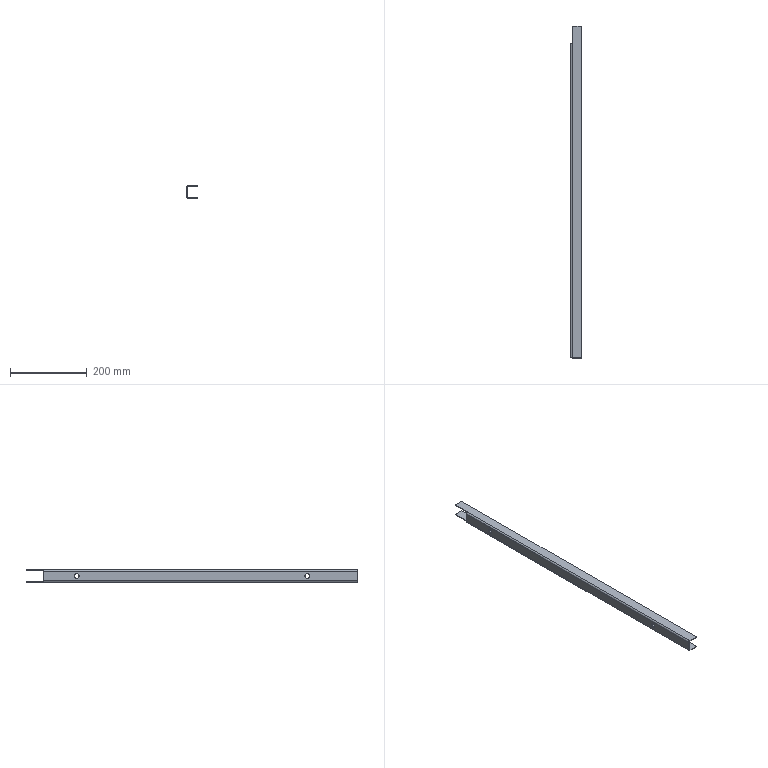Part | NX | features solid 2 | 1 solid | 28 faces | box 28 x 864.5 x 32 mm | volume 136877 mm3 | cylinder 14 | plane 14 | commonest cylinder face diameters 8 x8 12 x4 4 x2
STEP:
#1=CARTESIAN_POINT('',(1130.,-1461.75,470.));
#2=VERTEX_POINT('',#1);
#3=CARTESIAN_POINT('',(1130.,-1461.75,472.));
#4=VERTEX_POINT('',#3);
#5=CARTESIAN_POINT('',(1130.,-1461.75,1335.545));
#6=DIRECTION('',(0.,0.,-1.));
#7=VECTOR('',#6,1000.);
#8=LINE('',#5,#7);
#9=EDGE_CURVE('',#2,#4,#8,.F.);
#10=ORIENTED_EDGE('',*,*,#9,.T.);
#11=CARTESIAN_POINT('',(1130.,-1453.75,472.));
#12=VERTEX_POINT('',#11);
#13=CARTESIAN_POINT('',(1130.,-1457.75,472.));
#14=DIRECTION('',(0.,0.,-1.));
#15=DIRECTION('',(0.,1.,0.));
#16=AXIS2_PLACEMENT_3D('',#13,#14,#15);
#17=CIRCLE('',#16,4.);
#18=EDGE_CURVE('',#12,#4,#17,.T.);
#19=ORIENTED_EDGE('',*,*,#18,.F.);
#20=CARTESIAN_POINT('',(1130.,-1453.75,470.));
#21=VERTEX_POINT('',#20);
#22=CARTESIAN_POINT('',(1130.,-1453.75,1335.545));
#23=DIRECTION('',(0.,0.,-1.));
#24=VECTOR('',#23,1000.);
#25=LINE('',#22,#24);
#26=EDGE_CURVE('',#12,#21,#25,.T.);
#27=ORIENTED_EDGE('',*,*,#26,.T.);
#28=CARTESIAN_POINT('',(1130.,-1457.75,470.));
#29=DIRECTION('',(0.,0.,-1.));
#30=DIRECTION('',(0.,1.,0.));
#31=AXIS2_PLACEMENT_3D('',#28,#29,#30);
#32=CIRCLE('',#31,4.);
#33=EDGE_CURVE('',#21,#2,#32,.T.);
#34=ORIENTED_EDGE('',*,*,#33,.T.);
#35=EDGE_LOOP('',(#10,#19,#27,#34));
#36=FACE_BOUND('',#35,.T.);
#37=CARTESIAN_POINT('',(1130.,-1457.75,1335.545));
#38=DIRECTION('',(0.,0.,-1.));
#39=DIRECTION('',(0.,1.,0.));
#40=AXIS2_PLACEMENT_3D('',#37,#38,#39);
#41=CYLINDRICAL_SURFACE('',#40,4.);
#42=ADVANCED_FACE('',(#36),#41,.F.);
#43=CARTESIAN_POINT('',(1130.,-761.75,470.));
#44=VERTEX_POINT('',#43);
#45=CARTESIAN_POINT('',(1130.,-761.75,472.));
#46=VERTEX_POINT('',#45);
#47=CARTESIAN_POINT('',(1130.,-761.75,1335.545));
#48=DIRECTION('',(0.,0.,-1.));
#49=VECTOR('',#48,1000.);
#50=LINE('',#47,#49);
#51=EDGE_CURVE('',#44,#46,#50,.F.);
#52=ORIENTED_EDGE('',*,*,#51,.T.);
#53=CARTESIAN_POINT('',(1130.,-753.75,472.));
#54=VERTEX_POINT('',#53);
#55=CARTESIAN_POINT('',(1130.,-757.75,472.));
#56=DIRECTION('',(0.,0.,-1.));
#57=DIRECTION('',(0.,1.,0.));
#58=AXIS2_PLACEMENT_3D('',#55,#56,#57);
#59=CIRCLE('',#58,4.);
#60=EDGE_CURVE('',#54,#46,#59,.T.);
#61=ORIENTED_EDGE('',*,*,#60,.F.);
#62=CARTESIAN_POINT('',(1130.,-753.75,470.));
#63=VERTEX_POINT('',#62);
#64=CARTESIAN_POINT('',(1130.,-753.75,1335.545));
#65=DIRECTION('',(0.,0.,-1.));
#66=VECTOR('',#65,1000.);
#67=LINE('',#64,#66);
#68=EDGE_CURVE('',#54,#63,#67,.T.);
#69=ORIENTED_EDGE('',*,*,#68,.T.);
#70=CARTESIAN_POINT('',(1130.,-757.75,470.));
#71=DIRECTION('',(0.,0.,-1.));
#72=DIRECTION('',(0.,1.,0.));
#73=AXIS2_PLACEMENT_3D('',#70,#71,#72);
#74=CIRCLE('',#73,4.);
#75=EDGE_CURVE('',#63,#44,#74,.T.);
#76=ORIENTED_EDGE('',*,*,#75,.T.);
#77=EDGE_LOOP('',(#52,#61,#69,#76));
#78=FACE_BOUND('',#77,.T.);
#79=CARTESIAN_POINT('',(1130.,-757.75,1335.545));
#80=DIRECTION('',(0.,0.,-1.));
#81=DIRECTION('',(0.,1.,0.));
#82=AXIS2_PLACEMENT_3D('',#79,#80,#81);
#83=CYLINDRICAL_SURFACE('',#82,4.);
#84=ADVANCED_FACE('',(#78),#83,.F.);
#85=CARTESIAN_POINT('',(1130.,-1111.75,470.));
#86=VERTEX_POINT('',#85);
#87=CARTESIAN_POINT('',(1130.,-1111.75,472.));
#88=VERTEX_POINT('',#87);
#89=CARTESIAN_POINT('',(1130.,-1111.75,1335.545));
#90=DIRECTION('',(0.,0.,-1.));
#91=VECTOR('',#90,1000.);
#92=LINE('',#89,#91);
#93=EDGE_CURVE('',#86,#88,#92,.F.);
#94=ORIENTED_EDGE('',*,*,#93,.T.);
#95=CARTESIAN_POINT('',(1130.,-1103.75,472.));
#96=VERTEX_POINT('',#95);
#97=CARTESIAN_POINT('',(1130.,-1107.75,472.));
#98=DIRECTION('',(0.,0.,-1.));
#99=DIRECTION('',(0.,1.,0.));
#100=AXIS2_PLACEMENT_3D('',#97,#98,#99);
#101=CIRCLE('',#100,4.);
#102=EDGE_CURVE('',#96,#88,#101,.T.);
#103=ORIENTED_EDGE('',*,*,#102,.F.);
#104=CARTESIAN_POINT('',(1130.,-1103.75,470.));
#105=VERTEX_POINT('',#104);
#106=CARTESIAN_POINT('',(1130.,-1103.75,1335.545));
#107=DIRECTION('',(0.,0.,-1.));
#108=VECTOR('',#107,1000.);
#109=LINE('',#106,#108);
#110=EDGE_CURVE('',#96,#105,#109,.T.);
#111=ORIENTED_EDGE('',*,*,#110,.T.);
#112=CARTESIAN_POINT('',(1130.,-1107.75,470.));
#113=DIRECTION('',(0.,0.,-1.));
#114=DIRECTION('',(0.,1.,0.));
#115=AXIS2_PLACEMENT_3D('',#112,#113,#114);
#116=CIRCLE('',#115,4.);
#117=EDGE_CURVE('',#105,#86,#116,.T.);
#118=ORIENTED_EDGE('',*,*,#117,.T.);
#119=EDGE_LOOP('',(#94,#103,#111,#118));
#120=FACE_BOUND('',#119,.T.);
#121=CARTESIAN_POINT('',(1130.,-1107.75,1335.545));
#122=DIRECTION('',(0.,0.,-1.));
#123=DIRECTION('',(0.,1.,0.));
#124=AXIS2_PLACEMENT_3D('',#121,#122,#123);
#125=CYLINDRICAL_SURFACE('',#124,4.);
#126=ADVANCED_FACE('',(#120),#125,.F.);
#127=CARTESIAN_POINT('',(1110.,-807.75,492.));
#128=VERTEX_POINT('',#127);
#129=CARTESIAN_POINT('',(1112.,-807.75,492.));
#130=VERTEX_POINT('',#129);
#131=CARTESIAN_POINT('',(1975.545,-807.75,492.));
#132=DIRECTION('',(-1.,0.,0.));
#133=VECTOR('',#132,1000.);
#134=LINE('',#131,#133);
#135=EDGE_CURVE('',#128,#130,#134,.F.);
#136=ORIENTED_EDGE('',*,*,#135,.T.);
#137=CARTESIAN_POINT('',(1112.,-807.75,480.));
#138=VERTEX_POINT('',#137);
#139=CARTESIAN_POINT('',(1112.,-807.75,486.));
#140=DIRECTION('',(-1.,0.,0.));
#141=DIRECTION('',(0.,0.,-1.));
#142=AXIS2_PLACEMENT_3D('',#139,#140,#141);
#143=CIRCLE('',#142,6.);
#144=EDGE_CURVE('',#138,#130,#143,.T.);
#145=ORIENTED_EDGE('',*,*,#144,.F.);
#146=CARTESIAN_POINT('',(1110.,-807.75,480.));
#147=VERTEX_POINT('',#146);
#148=CARTESIAN_POINT('',(1975.545,-807.75,480.));
#149=DIRECTION('',(-1.,0.,0.));
#150=VECTOR('',#149,1000.);
#151=LINE('',#148,#150);
#152=EDGE_CURVE('',#138,#147,#151,.T.);
#153=ORIENTED_EDGE('',*,*,#152,.T.);
#154=CARTESIAN_POINT('',(1110.,-807.75,486.));
#155=DIRECTION('',(-1.,0.,0.));
#156=DIRECTION('',(0.,-1.,0.));
#157=AXIS2_PLACEMENT_3D('',#154,#155,#156);
#158=CIRCLE('',#157,6.);
#159=EDGE_CURVE('',#147,#128,#158,.T.);
#160=ORIENTED_EDGE('',*,*,#159,.T.);
#161=EDGE_LOOP('',(#136,#145,#153,#160));
#162=FACE_BOUND('',#161,.T.);
#163=CARTESIAN_POINT('',(1975.545,-807.75,486.));
#164=DIRECTION('',(-1.,0.,0.));
#165=DIRECTION('',(0.,0.,-1.));
#166=AXIS2_PLACEMENT_3D('',#163,#164,#165);
#167=CYLINDRICAL_SURFACE('',#166,6.);
#168=ADVANCED_FACE('',(#162),#167,.F.);
#169=CARTESIAN_POINT('',(1112.,-1407.75,492.));
#170=VERTEX_POINT('',#169);
#171=CARTESIAN_POINT('',(1110.,-1407.75,492.));
#172=VERTEX_POINT('',#171);
#173=CARTESIAN_POINT('',(1975.545,-1407.75,492.));
#174=DIRECTION('',(-1.,0.,0.));
#175=VECTOR('',#174,1000.);
#176=LINE('',#173,#175);
#177=EDGE_CURVE('',#170,#172,#176,.T.);
#178=ORIENTED_EDGE('',*,*,#177,.F.);
#179=CARTESIAN_POINT('',(1112.,-1407.75,480.));
#180=VERTEX_POINT('',#179);
#181=CARTESIAN_POINT('',(1112.,-1407.75,486.));
#182=DIRECTION('',(-1.,0.,0.));
#183=DIRECTION('',(0.,0.,-1.));
#184=AXIS2_PLACEMENT_3D('',#181,#182,#183);
#185=CIRCLE('',#184,6.);
#186=EDGE_CURVE('',#180,#170,#185,.T.);
#187=ORIENTED_EDGE('',*,*,#186,.F.);
#188=CARTESIAN_POINT('',(1110.,-1407.75,480.));
#189=VERTEX_POINT('',#188);
#190=CARTESIAN_POINT('',(1975.545,-1407.75,480.));
#191=DIRECTION('',(-1.,0.,0.));
#192=VECTOR('',#191,1000.);
#193=LINE('',#190,#192);
#194=EDGE_CURVE('',#189,#180,#193,.F.);
#195=ORIENTED_EDGE('',*,*,#194,.F.);
#196=CARTESIAN_POINT('',(1110.,-1407.75,486.));
#197=DIRECTION('',(-1.,0.,0.));
#198=DIRECTION('',(0.,-1.,0.));
#199=AXIS2_PLACEMENT_3D('',#196,#197,#198);
#200=CIRCLE('',#199,6.);
#201=EDGE_CURVE('',#189,#172,#200,.T.);
#202=ORIENTED_EDGE('',*,*,#201,.T.);
#203=EDGE_LOOP('',(#178,#187,#195,#202));
#204=FACE_BOUND('',#203,.T.);
#205=CARTESIAN_POINT('',(1975.545,-1407.75,486.));
#206=DIRECTION('',(-1.,0.,0.));
#207=DIRECTION('',(0.,0.,-1.));
#208=AXIS2_PLACEMENT_3D('',#205,#206,#207);
#209=CYLINDRICAL_SURFACE('',#208,6.);
#210=ADVANCED_FACE('',(#204),#209,.F.);
#211=CARTESIAN_POINT('',(1114.,-720.,500.));
#212=VERTEX_POINT('',#211);
#213=CARTESIAN_POINT('',(1112.,-720.,498.));
#214=VERTEX_POINT('',#213);
#215=CARTESIAN_POINT('',(1114.,-720.,498.));
#216=DIRECTION('',(0.,-1.,0.));
#217=DIRECTION('',(0.,0.,-1.));
#218=AXIS2_PLACEMENT_3D('',#215,#216,#217);
#219=CIRCLE('',#218,2.);
#220=EDGE_CURVE('',#212,#214,#219,.T.);
#221=ORIENTED_EDGE('',*,*,#220,.T.);
#222=CARTESIAN_POINT('',(1112.,-720.,474.));
#223=VERTEX_POINT('',#222);
#224=CARTESIAN_POINT('',(1112.,-720.,502.));
#225=DIRECTION('',(0.,0.,-1.));
#226=VECTOR('',#225,1000.);
#227=LINE('',#224,#226);
#228=EDGE_CURVE('',#214,#223,#227,.T.);
#229=ORIENTED_EDGE('',*,*,#228,.T.);
#230=CARTESIAN_POINT('',(1114.,-720.,472.));
#231=VERTEX_POINT('',#230);
#232=CARTESIAN_POINT('',(1114.,-720.,474.));
#233=DIRECTION('',(0.,-1.,0.));
#234=DIRECTION('',(0.,0.,-1.));
#235=AXIS2_PLACEMENT_3D('',#232,#233,#234);
#236=CIRCLE('',#235,2.);
#237=EDGE_CURVE('',#223,#231,#236,.T.);
#238=ORIENTED_EDGE('',*,*,#237,.T.);
#239=CARTESIAN_POINT('',(1115.,-720.,472.));
#240=VERTEX_POINT('',#239);
#241=CARTESIAN_POINT('',(1110.,-720.,472.));
#242=DIRECTION('',(1.,0.,0.));
#243=VECTOR('',#242,1000.);
#244=LINE('',#241,#243);
#245=EDGE_CURVE('',#231,#240,#244,.T.);
#246=ORIENTED_EDGE('',*,*,#245,.T.);
#247=CARTESIAN_POINT('',(1115.,-720.,470.));
#248=VERTEX_POINT('',#247);
#249=CARTESIAN_POINT('',(1115.,-720.,470.));
#250=DIRECTION('',(0.,0.,-1.));
#251=VECTOR('',#250,1000.);
#252=LINE('',#249,#251);
#253=EDGE_CURVE('',#240,#248,#252,.T.);
#254=ORIENTED_EDGE('',*,*,#253,.T.);
#255=CARTESIAN_POINT('',(1114.,-720.,470.));
#256=VERTEX_POINT('',#255);
#257=CARTESIAN_POINT('',(1110.,-720.,470.));
#258=DIRECTION('',(1.,0.,0.));
#259=VECTOR('',#258,1000.);
#260=LINE('',#257,#259);
#261=EDGE_CURVE('',#256,#248,#260,.T.);
#262=ORIENTED_EDGE('',*,*,#261,.F.);
#263=CARTESIAN_POINT('',(1110.,-720.,474.));
#264=VERTEX_POINT('',#263);
#265=CARTESIAN_POINT('',(1114.,-720.,474.));
#266=DIRECTION('',(0.,-1.,0.));
#267=DIRECTION('',(0.,0.,1.));
#268=AXIS2_PLACEMENT_3D('',#265,#266,#267);
#269=CIRCLE('',#268,4.);
#270=EDGE_CURVE('',#264,#256,#269,.T.);
#271=ORIENTED_EDGE('',*,*,#270,.F.);
#272=CARTESIAN_POINT('',(1110.,-720.,498.));
#273=VERTEX_POINT('',#272);
#274=CARTESIAN_POINT('',(1110.,-720.,502.));
#275=DIRECTION('',(0.,0.,-1.));
#276=VECTOR('',#275,1000.);
#277=LINE('',#274,#276);
#278=EDGE_CURVE('',#273,#264,#277,.T.);
#279=ORIENTED_EDGE('',*,*,#278,.F.);
#280=CARTESIAN_POINT('',(1114.,-720.,502.));
#281=VERTEX_POINT('',#280);
#282=CARTESIAN_POINT('',(1114.,-720.,498.));
#283=DIRECTION('',(0.,-1.,0.));
#284=DIRECTION('',(0.,0.,1.));
#285=AXIS2_PLACEMENT_3D('',#282,#283,#284);
#286=CIRCLE('',#285,4.);
#287=EDGE_CURVE('',#281,#273,#286,.T.);
#288=ORIENTED_EDGE('',*,*,#287,.F.);
#289=CARTESIAN_POINT('',(1115.,-720.,502.));
#290=VERTEX_POINT('',#289);
#291=CARTESIAN_POINT('',(1138.,-720.,502.));
#292=DIRECTION('',(-1.,0.,0.));
#293=VECTOR('',#292,1000.);
#294=LINE('',#291,#293);
#295=EDGE_CURVE('',#290,#281,#294,.T.);
#296=ORIENTED_EDGE('',*,*,#295,.F.);
#297=CARTESIAN_POINT('',(1115.,-720.,500.));
#298=VERTEX_POINT('',#297);
#299=CARTESIAN_POINT('',(1115.,-720.,502.));
#300=DIRECTION('',(0.,0.,1.));
#301=VECTOR('',#300,1000.);
#302=LINE('',#299,#301);
#303=EDGE_CURVE('',#298,#290,#302,.T.);
#304=ORIENTED_EDGE('',*,*,#303,.F.);
#305=CARTESIAN_POINT('',(1138.,-720.,500.));
#306=DIRECTION('',(-1.,0.,0.));
#307=VECTOR('',#306,1000.);
#308=LINE('',#305,#307);
#309=EDGE_CURVE('',#298,#212,#308,.T.);
#310=ORIENTED_EDGE('',*,*,#309,.T.);
#311=EDGE_LOOP('',(#221,#229,#238,#246,#254,#262,#271,#279,#288,#296,#304,#310));
#312=FACE_BOUND('',#311,.T.);
#313=CARTESIAN_POINT('',(1114.,-720.,498.));
#314=DIRECTION('',(0.,-1.,0.));
#315=DIRECTION('',(-1.,0.,0.));
#316=AXIS2_PLACEMENT_3D('',#313,#314,#315);
#317=PLANE('',#316);
#318=ADVANCED_FACE('',(#312),#317,.F.);
#319=CARTESIAN_POINT('',(1115.,-675.5,472.));
#320=VERTEX_POINT('',#319);
#321=CARTESIAN_POINT('',(1115.,-675.5,470.));
#322=VERTEX_POINT('',#321);
#323=CARTESIAN_POINT('',(1115.,-675.5,470.));
#324=DIRECTION('',(0.,0.,-1.));
#325=VECTOR('',#324,1000.);
#326=LINE('',#323,#325);
#327=EDGE_CURVE('',#320,#322,#326,.T.);
#328=ORIENTED_EDGE('',*,*,#327,.T.);
#329=CARTESIAN_POINT('',(1115.,-675.5,470.));
#330=DIRECTION('',(0.,1.,0.));
#331=VECTOR('',#330,1000.);
#332=LINE('',#329,#331);
#333=EDGE_CURVE('',#248,#322,#332,.T.);
#334=ORIENTED_EDGE('',*,*,#333,.F.);
#335=ORIENTED_EDGE('',*,*,#253,.F.);
#336=CARTESIAN_POINT('',(1115.,-675.5,472.));
#337=DIRECTION('',(0.,1.,0.));
#338=VECTOR('',#337,1000.);
#339=LINE('',#336,#338);
#340=EDGE_CURVE('',#240,#320,#339,.T.);
#341=ORIENTED_EDGE('',*,*,#340,.T.);
#342=EDGE_LOOP('',(#328,#334,#335,#341));
#343=FACE_BOUND('',#342,.T.);
#344=CARTESIAN_POINT('',(1115.,-675.5,470.));
#345=DIRECTION('',(-1.,0.,0.));
#346=DIRECTION('',(0.,0.,1.));
#347=AXIS2_PLACEMENT_3D('',#344,#345,#346);
#348=PLANE('',#347);
#349=ADVANCED_FACE('',(#343),#348,.T.);
#350=ORIENTED_EDGE('',*,*,#303,.T.);
#351=CARTESIAN_POINT('',(1115.,-675.5,502.));
#352=VERTEX_POINT('',#351);
#353=CARTESIAN_POINT('',(1115.,-675.5,502.));
#354=DIRECTION('',(0.,-1.,0.));
#355=VECTOR('',#354,1000.);
#356=LINE('',#353,#355);
#357=EDGE_CURVE('',#352,#290,#356,.T.);
#358=ORIENTED_EDGE('',*,*,#357,.F.);
#359=CARTESIAN_POINT('',(1115.,-675.5,500.));
#360=VERTEX_POINT('',#359);
#361=CARTESIAN_POINT('',(1115.,-675.5,502.));
#362=DIRECTION('',(0.,0.,1.));
#363=VECTOR('',#362,1000.);
#364=LINE('',#361,#363);
#365=EDGE_CURVE('',#360,#352,#364,.T.);
#366=ORIENTED_EDGE('',*,*,#365,.F.);
#367=CARTESIAN_POINT('',(1115.,-675.5,500.));
#368=DIRECTION('',(0.,-1.,0.));
#369=VECTOR('',#368,1000.);
#370=LINE('',#367,#369);
#371=EDGE_CURVE('',#360,#298,#370,.T.);
#372=ORIENTED_EDGE('',*,*,#371,.T.);
#373=EDGE_LOOP('',(#350,#358,#366,#372));
#374=FACE_BOUND('',#373,.T.);
#375=CARTESIAN_POINT('',(1115.,-675.5,502.));
#376=DIRECTION('',(-1.,0.,0.));
#377=DIRECTION('',(0.,0.,1.));
#378=AXIS2_PLACEMENT_3D('',#375,#376,#377);
#379=PLANE('',#378);
#380=ADVANCED_FACE('',(#374),#379,.T.);
#381=ORIENTED_EDGE('',*,*,#102,.T.);
#382=CARTESIAN_POINT('',(1130.,-1107.75,472.));
#383=DIRECTION('',(0.,0.,-1.));
#384=DIRECTION('',(0.,1.,0.));
#385=AXIS2_PLACEMENT_3D('',#382,#383,#384);
#386=CIRCLE('',#385,4.);
#387=EDGE_CURVE('',#88,#96,#386,.T.);
#388=ORIENTED_EDGE('',*,*,#387,.T.);
#389=EDGE_LOOP('',(#381,#388));
#390=FACE_BOUND('',#389,.T.);
#391=ORIENTED_EDGE('',*,*,#60,.T.);
#392=CARTESIAN_POINT('',(1130.,-757.75,472.));
#393=DIRECTION('',(0.,0.,-1.));
#394=DIRECTION('',(0.,1.,0.));
#395=AXIS2_PLACEMENT_3D('',#392,#393,#394);
#396=CIRCLE('',#395,4.);
#397=EDGE_CURVE('',#46,#54,#396,.T.);
#398=ORIENTED_EDGE('',*,*,#397,.T.);
#399=EDGE_LOOP('',(#391,#398));
#400=FACE_BOUND('',#399,.T.);
#401=ORIENTED_EDGE('',*,*,#18,.T.);
#402=CARTESIAN_POINT('',(1130.,-1457.75,472.));
#403=DIRECTION('',(0.,0.,-1.));
#404=DIRECTION('',(0.,1.,0.));
#405=AXIS2_PLACEMENT_3D('',#402,#403,#404);
#406=CIRCLE('',#405,4.);
#407=EDGE_CURVE('',#4,#12,#406,.T.);
#408=ORIENTED_EDGE('',*,*,#407,.T.);
#409=EDGE_LOOP('',(#401,#408));
#410=FACE_BOUND('',#409,.T.);
#411=CARTESIAN_POINT('',(1138.,-675.5,472.));
#412=VERTEX_POINT('',#411);
#413=CARTESIAN_POINT('',(1110.,-675.5,472.));
#414=DIRECTION('',(1.,0.,0.));
#415=VECTOR('',#414,1000.);
#416=LINE('',#413,#415);
#417=EDGE_CURVE('',#320,#412,#416,.T.);
#418=ORIENTED_EDGE('',*,*,#417,.F.);
#419=ORIENTED_EDGE('',*,*,#340,.F.);
#420=ORIENTED_EDGE('',*,*,#245,.F.);
#421=CARTESIAN_POINT('',(1114.,-1540.,472.));
#422=VERTEX_POINT('',#421);
#423=CARTESIAN_POINT('',(1114.,-675.5,472.));
#424=DIRECTION('',(0.,-1.,0.));
#425=VECTOR('',#424,1000.);
#426=LINE('',#423,#425);
#427=EDGE_CURVE('',#231,#422,#426,.T.);
#428=ORIENTED_EDGE('',*,*,#427,.T.);
#429=CARTESIAN_POINT('',(1138.,-1540.,472.));
#430=VERTEX_POINT('',#429);
#431=CARTESIAN_POINT('',(1110.,-1540.,472.));
#432=DIRECTION('',(1.,0.,0.));
#433=VECTOR('',#432,1000.);
#434=LINE('',#431,#433);
#435=EDGE_CURVE('',#422,#430,#434,.T.);
#436=ORIENTED_EDGE('',*,*,#435,.T.);
#437=CARTESIAN_POINT('',(1138.,-675.5,472.));
#438=DIRECTION('',(0.,-1.,0.));
#439=VECTOR('',#438,1000.);
#440=LINE('',#437,#439);
#441=EDGE_CURVE('',#412,#430,#440,.T.);
#442=ORIENTED_EDGE('',*,*,#441,.F.);
#443=EDGE_LOOP('',(#418,#419,#420,#428,#436,#442));
#444=FACE_BOUND('',#443,.T.);
#445=CARTESIAN_POINT('',(1110.,-675.5,472.));
#446=DIRECTION('',(0.,0.,-1.));
#447=DIRECTION('',(0.,-1.,0.));
#448=AXIS2_PLACEMENT_3D('',#445,#446,#447);
#449=PLANE('',#448);
#450=ADVANCED_FACE('',(#390,#400,#410,#444),#449,.F.);
#451=ORIENTED_EDGE('',*,*,#427,.F.);
#452=ORIENTED_EDGE('',*,*,#237,.F.);
#453=CARTESIAN_POINT('',(1112.,-1540.,474.));
#454=VERTEX_POINT('',#453);
#455=CARTESIAN_POINT('',(1112.,-675.5,474.));
#456=DIRECTION('',(0.,-1.,0.));
#457=VECTOR('',#456,1000.);
#458=LINE('',#455,#457);
#459=EDGE_CURVE('',#223,#454,#458,.T.);
#460=ORIENTED_EDGE('',*,*,#459,.T.);
#461=CARTESIAN_POINT('',(1114.,-1540.,474.));
#462=DIRECTION('',(0.,-1.,0.));
#463=DIRECTION('',(0.,0.,-1.));
#464=AXIS2_PLACEMENT_3D('',#461,#462,#463);
#465=CIRCLE('',#464,2.);
#466=EDGE_CURVE('',#454,#422,#465,.T.);
#467=ORIENTED_EDGE('',*,*,#466,.T.);
#468=EDGE_LOOP('',(#451,#452,#460,#467));
#469=FACE_BOUND('',#468,.T.);
#470=CARTESIAN_POINT('',(1114.,-675.5,474.));
#471=DIRECTION('',(0.,-1.,0.));
#472=DIRECTION('',(0.,0.,-1.));
#473=AXIS2_PLACEMENT_3D('',#470,#471,#472);
#474=CYLINDRICAL_SURFACE('',#473,2.);
#475=ADVANCED_FACE('',(#469),#474,.F.);
#476=ORIENTED_EDGE('',*,*,#186,.T.);
#477=CARTESIAN_POINT('',(1112.,-1407.75,486.));
#478=DIRECTION('',(-1.,0.,0.));
#479=DIRECTION('',(0.,0.,-1.));
#480=AXIS2_PLACEMENT_3D('',#477,#478,#479);
#481=CIRCLE('',#480,6.);
#482=EDGE_CURVE('',#170,#180,#481,.T.);
#483=ORIENTED_EDGE('',*,*,#482,.T.);
#484=EDGE_LOOP('',(#476,#483));
#485=FACE_BOUND('',#484,.T.);
#486=ORIENTED_EDGE('',*,*,#144,.T.);
#487=CARTESIAN_POINT('',(1112.,-807.75,486.));
#488=DIRECTION('',(-1.,0.,0.));
#489=DIRECTION('',(0.,0.,-1.));
#490=AXIS2_PLACEMENT_3D('',#487,#488,#489);
#491=CIRCLE('',#490,6.);
#492=EDGE_CURVE('',#130,#138,#491,.T.);
#493=ORIENTED_EDGE('',*,*,#492,.T.);
#494=EDGE_LOOP('',(#486,#493));
#495=FACE_BOUND('',#494,.T.);
#496=ORIENTED_EDGE('',*,*,#459,.F.);
#497=ORIENTED_EDGE('',*,*,#228,.F.);
#498=CARTESIAN_POINT('',(1112.,-1540.,498.));
#499=VERTEX_POINT('',#498);
#500=CARTESIAN_POINT('',(1112.,-675.5,498.));
#501=DIRECTION('',(0.,-1.,0.));
#502=VECTOR('',#501,1000.);
#503=LINE('',#500,#502);
#504=EDGE_CURVE('',#214,#499,#503,.T.);
#505=ORIENTED_EDGE('',*,*,#504,.T.);
#506=CARTESIAN_POINT('',(1112.,-1540.,502.));
#507=DIRECTION('',(0.,0.,-1.));
#508=VECTOR('',#507,1000.);
#509=LINE('',#506,#508);
#510=EDGE_CURVE('',#499,#454,#509,.T.);
#511=ORIENTED_EDGE('',*,*,#510,.T.);
#512=EDGE_LOOP('',(#496,#497,#505,#511));
#513=FACE_BOUND('',#512,.T.);
#514=CARTESIAN_POINT('',(1112.,-675.5,502.));
#515=DIRECTION('',(-1.,0.,0.));
#516=DIRECTION('',(0.,0.,1.));
#517=AXIS2_PLACEMENT_3D('',#514,#515,#516);
#518=PLANE('',#517);
#519=ADVANCED_FACE('',(#485,#495,#513),#518,.F.);
#520=ORIENTED_EDGE('',*,*,#504,.F.);
#521=ORIENTED_EDGE('',*,*,#220,.F.);
#522=CARTESIAN_POINT('',(1114.,-1540.,500.));
#523=VERTEX_POINT('',#522);
#524=CARTESIAN_POINT('',(1114.,-675.5,500.));
#525=DIRECTION('',(0.,-1.,0.));
#526=VECTOR('',#525,1000.);
#527=LINE('',#524,#526);
#528=EDGE_CURVE('',#212,#523,#527,.T.);
#529=ORIENTED_EDGE('',*,*,#528,.T.);
#530=CARTESIAN_POINT('',(1114.,-1540.,498.));
#531=DIRECTION('',(0.,-1.,0.));
#532=DIRECTION('',(0.,0.,-1.));
#533=AXIS2_PLACEMENT_3D('',#530,#531,#532);
#534=CIRCLE('',#533,2.);
#535=EDGE_CURVE('',#523,#499,#534,.T.);
#536=ORIENTED_EDGE('',*,*,#535,.T.);
#537=EDGE_LOOP('',(#520,#521,#529,#536));
#538=FACE_BOUND('',#537,.T.);
#539=CARTESIAN_POINT('',(1114.,-675.5,498.));
#540=DIRECTION('',(0.,-1.,0.));
#541=DIRECTION('',(0.,0.,-1.));
#542=AXIS2_PLACEMENT_3D('',#539,#540,#541);
#543=CYLINDRICAL_SURFACE('',#542,2.);
#544=ADVANCED_FACE('',(#538),#543,.F.);
#545=ORIENTED_EDGE('',*,*,#309,.F.);
#546=ORIENTED_EDGE('',*,*,#371,.F.);
#547=CARTESIAN_POINT('',(1138.,-675.5,500.));
#548=VERTEX_POINT('',#547);
#549=CARTESIAN_POINT('',(1138.,-675.5,500.));
#550=DIRECTION('',(-1.,0.,0.));
#551=VECTOR('',#550,1000.);
#552=LINE('',#549,#551);
#553=EDGE_CURVE('',#548,#360,#552,.T.);
#554=ORIENTED_EDGE('',*,*,#553,.F.);
#555=CARTESIAN_POINT('',(1138.,-1540.,500.));
#556=VERTEX_POINT('',#555);
#557=CARTESIAN_POINT('',(1138.,-675.5,500.));
#558=DIRECTION('',(0.,-1.,0.));
#559=VECTOR('',#558,1000.);
#560=LINE('',#557,#559);
#561=EDGE_CURVE('',#548,#556,#560,.T.);
#562=ORIENTED_EDGE('',*,*,#561,.T.);
#563=CARTESIAN_POINT('',(1138.,-1540.,500.));
#564=DIRECTION('',(-1.,0.,0.));
#565=VECTOR('',#564,1000.);
#566=LINE('',#563,#565);
#567=EDGE_CURVE('',#556,#523,#566,.T.);
#568=ORIENTED_EDGE('',*,*,#567,.T.);
#569=ORIENTED_EDGE('',*,*,#528,.F.);
#570=EDGE_LOOP('',(#545,#546,#554,#562,#568,#569));
#571=FACE_BOUND('',#570,.T.);
#572=CARTESIAN_POINT('',(1138.,-675.5,500.));
#573=DIRECTION('',(0.,0.,1.));
#574=DIRECTION('',(1.,0.,0.));
#575=AXIS2_PLACEMENT_3D('',#572,#573,#574);
#576=PLANE('',#575);
#577=ADVANCED_FACE('',(#571),#576,.F.);
#578=ORIENTED_EDGE('',*,*,#117,.F.);
#579=CARTESIAN_POINT('',(1130.,-1107.75,470.));
#580=DIRECTION('',(0.,0.,-1.));
#581=DIRECTION('',(0.,1.,0.));
#582=AXIS2_PLACEMENT_3D('',#579,#580,#581);
#583=CIRCLE('',#582,4.);
#584=EDGE_CURVE('',#86,#105,#583,.T.);
#585=ORIENTED_EDGE('',*,*,#584,.F.);
#586=EDGE_LOOP('',(#578,#585));
#587=FACE_BOUND('',#586,.T.);
#588=ORIENTED_EDGE('',*,*,#75,.F.);
#589=CARTESIAN_POINT('',(1130.,-757.75,470.));
#590=DIRECTION('',(0.,0.,-1.));
#591=DIRECTION('',(0.,1.,0.));
#592=AXIS2_PLACEMENT_3D('',#589,#590,#591);
#593=CIRCLE('',#592,4.);
#594=EDGE_CURVE('',#44,#63,#593,.T.);
#595=ORIENTED_EDGE('',*,*,#594,.F.);
#596=EDGE_LOOP('',(#588,#595));
#597=FACE_BOUND('',#596,.T.);
#598=ORIENTED_EDGE('',*,*,#33,.F.);
#599=CARTESIAN_POINT('',(1130.,-1457.75,470.));
#600=DIRECTION('',(0.,0.,-1.));
#601=DIRECTION('',(0.,1.,0.));
#602=AXIS2_PLACEMENT_3D('',#599,#600,#601);
#603=CIRCLE('',#602,4.);
#604=EDGE_CURVE('',#2,#21,#603,.T.);
#605=ORIENTED_EDGE('',*,*,#604,.F.);
#606=EDGE_LOOP('',(#598,#605));
#607=FACE_BOUND('',#606,.T.);
#608=ORIENTED_EDGE('',*,*,#333,.T.);
#609=CARTESIAN_POINT('',(1138.,-675.5,470.));
#610=VERTEX_POINT('',#609);
#611=CARTESIAN_POINT('',(1110.,-675.5,470.));
#612=DIRECTION('',(1.,0.,0.));
#613=VECTOR('',#612,1000.);
#614=LINE('',#611,#613);
#615=EDGE_CURVE('',#322,#610,#614,.T.);
#616=ORIENTED_EDGE('',*,*,#615,.T.);
#617=CARTESIAN_POINT('',(1138.,-1540.,470.));
#618=VERTEX_POINT('',#617);
#619=CARTESIAN_POINT('',(1138.,-675.5,470.));
#620=DIRECTION('',(0.,-1.,0.));
#621=VECTOR('',#620,1000.);
#622=LINE('',#619,#621);
#623=EDGE_CURVE('',#610,#618,#622,.T.);
#624=ORIENTED_EDGE('',*,*,#623,.T.);
#625=CARTESIAN_POINT('',(1114.,-1540.,470.));
#626=VERTEX_POINT('',#625);
#627=CARTESIAN_POINT('',(1110.,-1540.,470.));
#628=DIRECTION('',(1.,0.,0.));
#629=VECTOR('',#628,1000.);
#630=LINE('',#627,#629);
#631=EDGE_CURVE('',#626,#618,#630,.T.);
#632=ORIENTED_EDGE('',*,*,#631,.F.);
#633=CARTESIAN_POINT('',(1114.,-675.5,470.));
#634=DIRECTION('',(0.,-1.,0.));
#635=VECTOR('',#634,1000.);
#636=LINE('',#633,#635);
#637=EDGE_CURVE('',#256,#626,#636,.T.);
#638=ORIENTED_EDGE('',*,*,#637,.F.);
#639=ORIENTED_EDGE('',*,*,#261,.T.);
#640=EDGE_LOOP('',(#608,#616,#624,#632,#638,#639));
#641=FACE_BOUND('',#640,.T.);
#642=CARTESIAN_POINT('',(1110.,-675.5,470.));
#643=DIRECTION('',(0.,0.,-1.));
#644=DIRECTION('',(0.,-1.,0.));
#645=AXIS2_PLACEMENT_3D('',#642,#643,#644);
#646=PLANE('',#645);
#647=ADVANCED_FACE('',(#587,#597,#607,#641),#646,.T.);
#648=ORIENTED_EDGE('',*,*,#270,.T.);
#649=ORIENTED_EDGE('',*,*,#637,.T.);
#650=CARTESIAN_POINT('',(1110.,-1540.,474.));
#651=VERTEX_POINT('',#650);
#652=CARTESIAN_POINT('',(1114.,-1540.,474.));
#653=DIRECTION('',(0.,-1.,0.));
#654=DIRECTION('',(-1.,0.,0.));
#655=AXIS2_PLACEMENT_3D('',#652,#653,#654);
#656=CIRCLE('',#655,4.);
#657=EDGE_CURVE('',#651,#626,#656,.T.);
#658=ORIENTED_EDGE('',*,*,#657,.F.);
#659=CARTESIAN_POINT('',(1110.,-675.5,474.));
#660=DIRECTION('',(0.,-1.,0.));
#661=VECTOR('',#660,1000.);
#662=LINE('',#659,#661);
#663=EDGE_CURVE('',#264,#651,#662,.T.);
#664=ORIENTED_EDGE('',*,*,#663,.F.);
#665=EDGE_LOOP('',(#648,#649,#658,#664));
#666=FACE_BOUND('',#665,.T.);
#667=CARTESIAN_POINT('',(1114.,-675.5,474.));
#668=DIRECTION('',(0.,-1.,0.));
#669=DIRECTION('',(0.,0.,-1.));
#670=AXIS2_PLACEMENT_3D('',#667,#668,#669);
#671=CYLINDRICAL_SURFACE('',#670,4.);
#672=ADVANCED_FACE('',(#666),#671,.T.);
#673=ORIENTED_EDGE('',*,*,#201,.F.);
#674=CARTESIAN_POINT('',(1110.,-1407.75,486.));
#675=DIRECTION('',(-1.,0.,0.));
#676=DIRECTION('',(0.,-1.,0.));
#677=AXIS2_PLACEMENT_3D('',#674,#675,#676);
#678=CIRCLE('',#677,6.);
#679=EDGE_CURVE('',#172,#189,#678,.T.);
#680=ORIENTED_EDGE('',*,*,#679,.F.);
#681=EDGE_LOOP('',(#673,#680));
#682=FACE_BOUND('',#681,.T.);
#683=ORIENTED_EDGE('',*,*,#159,.F.);
#684=CARTESIAN_POINT('',(1110.,-807.75,486.));
#685=DIRECTION('',(-1.,0.,0.));
#686=DIRECTION('',(0.,-1.,0.));
#687=AXIS2_PLACEMENT_3D('',#684,#685,#686);
#688=CIRCLE('',#687,6.);
#689=EDGE_CURVE('',#128,#147,#688,.T.);
#690=ORIENTED_EDGE('',*,*,#689,.F.);
#691=EDGE_LOOP('',(#683,#690));
#692=FACE_BOUND('',#691,.T.);
#693=ORIENTED_EDGE('',*,*,#278,.T.);
#694=ORIENTED_EDGE('',*,*,#663,.T.);
#695=CARTESIAN_POINT('',(1110.,-1540.,498.));
#696=VERTEX_POINT('',#695);
#697=CARTESIAN_POINT('',(1110.,-1540.,502.));
#698=DIRECTION('',(0.,0.,-1.));
#699=VECTOR('',#698,1000.);
#700=LINE('',#697,#699);
#701=EDGE_CURVE('',#696,#651,#700,.T.);
#702=ORIENTED_EDGE('',*,*,#701,.F.);
#703=CARTESIAN_POINT('',(1110.,-675.5,498.));
#704=DIRECTION('',(0.,-1.,0.));
#705=VECTOR('',#704,1000.);
#706=LINE('',#703,#705);
#707=EDGE_CURVE('',#273,#696,#706,.T.);
#708=ORIENTED_EDGE('',*,*,#707,.F.);
#709=EDGE_LOOP('',(#693,#694,#702,#708));
#710=FACE_BOUND('',#709,.T.);
#711=CARTESIAN_POINT('',(1110.,-675.5,502.));
#712=DIRECTION('',(-1.,0.,0.));
#713=DIRECTION('',(0.,0.,1.));
#714=AXIS2_PLACEMENT_3D('',#711,#712,#713);
#715=PLANE('',#714);
#716=ADVANCED_FACE('',(#682,#692,#710),#715,.T.);
#717=ORIENTED_EDGE('',*,*,#287,.T.);
#718=ORIENTED_EDGE('',*,*,#707,.T.);
#719=CARTESIAN_POINT('',(1114.,-1540.,502.));
#720=VERTEX_POINT('',#719);
#721=CARTESIAN_POINT('',(1114.,-1540.,498.));
#722=DIRECTION('',(0.,-1.,0.));
#723=DIRECTION('',(-1.,0.,0.));
#724=AXIS2_PLACEMENT_3D('',#721,#722,#723);
#725=CIRCLE('',#724,4.);
#726=EDGE_CURVE('',#720,#696,#725,.T.);
#727=ORIENTED_EDGE('',*,*,#726,.F.);
#728=CARTESIAN_POINT('',(1114.,-675.5,502.));
#729=DIRECTION('',(0.,-1.,0.));
#730=VECTOR('',#729,1000.);
#731=LINE('',#728,#730);
#732=EDGE_CURVE('',#281,#720,#731,.T.);
#733=ORIENTED_EDGE('',*,*,#732,.F.);
#734=EDGE_LOOP('',(#717,#718,#727,#733));
#735=FACE_BOUND('',#734,.T.);
#736=CARTESIAN_POINT('',(1114.,-675.5,498.));
#737=DIRECTION('',(0.,-1.,0.));
#738=DIRECTION('',(0.,0.,-1.));
#739=AXIS2_PLACEMENT_3D('',#736,#737,#738);
#740=CYLINDRICAL_SURFACE('',#739,4.);
#741=ADVANCED_FACE('',(#735),#740,.T.);
#742=ORIENTED_EDGE('',*,*,#357,.T.);
#743=ORIENTED_EDGE('',*,*,#295,.T.);
#744=ORIENTED_EDGE('',*,*,#732,.T.);
#745=CARTESIAN_POINT('',(1138.,-1540.,502.));
#746=VERTEX_POINT('',#745);
#747=CARTESIAN_POINT('',(1138.,-1540.,502.));
#748=DIRECTION('',(-1.,0.,0.));
#749=VECTOR('',#748,1000.);
#750=LINE('',#747,#749);
#751=EDGE_CURVE('',#746,#720,#750,.T.);
#752=ORIENTED_EDGE('',*,*,#751,.F.);
#753=CARTESIAN_POINT('',(1138.,-675.5,502.));
#754=VERTEX_POINT('',#753);
#755=CARTESIAN_POINT('',(1138.,-675.5,502.));
#756=DIRECTION('',(0.,-1.,0.));
#757=VECTOR('',#756,1000.);
#758=LINE('',#755,#757);
#759=EDGE_CURVE('',#754,#746,#758,.T.);
#760=ORIENTED_EDGE('',*,*,#759,.F.);
#761=CARTESIAN_POINT('',(1138.,-675.5,502.));
#762=DIRECTION('',(-1.,0.,0.));
#763=VECTOR('',#762,1000.);
#764=LINE('',#761,#763);
#765=EDGE_CURVE('',#754,#352,#764,.T.);
#766=ORIENTED_EDGE('',*,*,#765,.T.);
#767=EDGE_LOOP('',(#742,#743,#744,#752,#760,#766));
#768=FACE_BOUND('',#767,.T.);
#769=CARTESIAN_POINT('',(1138.,-675.5,502.));
#770=DIRECTION('',(0.,0.,1.));
#771=DIRECTION('',(1.,0.,0.));
#772=AXIS2_PLACEMENT_3D('',#769,#770,#771);
#773=PLANE('',#772);
#774=ADVANCED_FACE('',(#768),#773,.T.);
#775=ORIENTED_EDGE('',*,*,#561,.F.);
#776=CARTESIAN_POINT('',(1138.,-675.5,502.));
#777=DIRECTION('',(0.,0.,1.));
#778=VECTOR('',#777,1000.);
#779=LINE('',#776,#778);
#780=EDGE_CURVE('',#548,#754,#779,.T.);
#781=ORIENTED_EDGE('',*,*,#780,.T.);
#782=ORIENTED_EDGE('',*,*,#759,.T.);
#783=CARTESIAN_POINT('',(1138.,-1540.,502.));
#784=DIRECTION('',(0.,0.,1.));
#785=VECTOR('',#784,1000.);
#786=LINE('',#783,#785);
#787=EDGE_CURVE('',#556,#746,#786,.T.);
#788=ORIENTED_EDGE('',*,*,#787,.F.);
#789=EDGE_LOOP('',(#775,#781,#782,#788));
#790=FACE_BOUND('',#789,.T.);
#791=CARTESIAN_POINT('',(1138.,-675.5,502.));
#792=DIRECTION('',(-1.,0.,0.));
#793=DIRECTION('',(0.,0.,1.));
#794=AXIS2_PLACEMENT_3D('',#791,#792,#793);
#795=PLANE('',#794);
#796=ADVANCED_FACE('',(#790),#795,.F.);
#797=ORIENTED_EDGE('',*,*,#751,.T.);
#798=ORIENTED_EDGE('',*,*,#726,.T.);
#799=ORIENTED_EDGE('',*,*,#701,.T.);
#800=ORIENTED_EDGE('',*,*,#657,.T.);
#801=ORIENTED_EDGE('',*,*,#631,.T.);
#802=CARTESIAN_POINT('',(1138.,-1540.,470.));
#803=DIRECTION('',(0.,0.,-1.));
#804=VECTOR('',#803,1000.);
#805=LINE('',#802,#804);
#806=EDGE_CURVE('',#430,#618,#805,.T.);
#807=ORIENTED_EDGE('',*,*,#806,.F.);
#808=ORIENTED_EDGE('',*,*,#435,.F.);
#809=ORIENTED_EDGE('',*,*,#466,.F.);
#810=ORIENTED_EDGE('',*,*,#510,.F.);
#811=ORIENTED_EDGE('',*,*,#535,.F.);
#812=ORIENTED_EDGE('',*,*,#567,.F.);
#813=ORIENTED_EDGE('',*,*,#787,.T.);
#814=EDGE_LOOP('',(#797,#798,#799,#800,#801,#807,#808,#809,#810,#811,#812,#813));
#815=FACE_BOUND('',#814,.T.);
#816=CARTESIAN_POINT('',(1138.,-1540.,502.));
#817=DIRECTION('',(0.,1.,0.));
#818=DIRECTION('',(0.,0.,-1.));
#819=AXIS2_PLACEMENT_3D('',#816,#817,#818);
#820=PLANE('',#819);
#821=ADVANCED_FACE('',(#815),#820,.F.);
#822=CARTESIAN_POINT('',(1138.,-675.5,470.));
#823=DIRECTION('',(0.,0.,-1.));
#824=VECTOR('',#823,1000.);
#825=LINE('',#822,#824);
#826=EDGE_CURVE('',#412,#610,#825,.T.);
#827=ORIENTED_EDGE('',*,*,#826,.F.);
#828=ORIENTED_EDGE('',*,*,#441,.T.);
#829=ORIENTED_EDGE('',*,*,#806,.T.);
#830=ORIENTED_EDGE('',*,*,#623,.F.);
#831=EDGE_LOOP('',(#827,#828,#829,#830));
#832=FACE_BOUND('',#831,.T.);
#833=CARTESIAN_POINT('',(1138.,-675.5,470.));
#834=DIRECTION('',(1.,0.,0.));
#835=DIRECTION('',(0.,0.,1.));
#836=AXIS2_PLACEMENT_3D('',#833,#834,#835);
#837=PLANE('',#836);
#838=ADVANCED_FACE('',(#832),#837,.T.);
#839=ORIENTED_EDGE('',*,*,#327,.F.);
#840=ORIENTED_EDGE('',*,*,#417,.T.);
#841=ORIENTED_EDGE('',*,*,#826,.T.);
#842=ORIENTED_EDGE('',*,*,#615,.F.);
#843=EDGE_LOOP('',(#839,#840,#841,#842));
#844=FACE_BOUND('',#843,.T.);
#845=CARTESIAN_POINT('',(1110.,-675.5,470.));
#846=DIRECTION('',(0.,1.,0.));
#847=DIRECTION('',(0.,0.,-1.));
#848=AXIS2_PLACEMENT_3D('',#845,#846,#847);
#849=PLANE('',#848);
#850=ADVANCED_FACE('',(#844),#849,.T.);
#851=ORIENTED_EDGE('',*,*,#553,.T.);
#852=ORIENTED_EDGE('',*,*,#365,.T.);
#853=ORIENTED_EDGE('',*,*,#765,.F.);
#854=ORIENTED_EDGE('',*,*,#780,.F.);
#855=EDGE_LOOP('',(#851,#852,#853,#854));
#856=FACE_BOUND('',#855,.T.);
#857=CARTESIAN_POINT('',(1110.,-675.5,470.));
#858=DIRECTION('',(0.,1.,0.));
#859=DIRECTION('',(0.,0.,-1.));
#860=AXIS2_PLACEMENT_3D('',#857,#858,#859);
#861=PLANE('',#860);
#862=ADVANCED_FACE('',(#856),#861,.T.);
#863=ORIENTED_EDGE('',*,*,#482,.F.);
#864=ORIENTED_EDGE('',*,*,#177,.T.);
#865=ORIENTED_EDGE('',*,*,#679,.T.);
#866=ORIENTED_EDGE('',*,*,#194,.T.);
#867=EDGE_LOOP('',(#863,#864,#865,#866));
#868=FACE_BOUND('',#867,.T.);
#869=CARTESIAN_POINT('',(1975.545,-1407.75,486.));
#870=DIRECTION('',(-1.,0.,0.));
#871=DIRECTION('',(0.,0.,-1.));
#872=AXIS2_PLACEMENT_3D('',#869,#870,#871);
#873=CYLINDRICAL_SURFACE('',#872,6.);
#874=ADVANCED_FACE('',(#868),#873,.F.);
#875=ORIENTED_EDGE('',*,*,#492,.F.);
#876=ORIENTED_EDGE('',*,*,#135,.F.);
#877=ORIENTED_EDGE('',*,*,#689,.T.);
#878=ORIENTED_EDGE('',*,*,#152,.F.);
#879=EDGE_LOOP('',(#875,#876,#877,#878));
#880=FACE_BOUND('',#879,.T.);
#881=CARTESIAN_POINT('',(1975.545,-807.75,486.));
#882=DIRECTION('',(-1.,0.,0.));
#883=DIRECTION('',(0.,0.,-1.));
#884=AXIS2_PLACEMENT_3D('',#881,#882,#883);
#885=CYLINDRICAL_SURFACE('',#884,6.);
#886=ADVANCED_FACE('',(#880),#885,.F.);
#887=ORIENTED_EDGE('',*,*,#387,.F.);
#888=ORIENTED_EDGE('',*,*,#93,.F.);
#889=ORIENTED_EDGE('',*,*,#584,.T.);
#890=ORIENTED_EDGE('',*,*,#110,.F.);
#891=EDGE_LOOP('',(#887,#888,#889,#890));
#892=FACE_BOUND('',#891,.T.);
#893=CARTESIAN_POINT('',(1130.,-1107.75,1335.545));
#894=DIRECTION('',(0.,0.,-1.));
#895=DIRECTION('',(0.,1.,0.));
#896=AXIS2_PLACEMENT_3D('',#893,#894,#895);
#897=CYLINDRICAL_SURFACE('',#896,4.);
#898=ADVANCED_FACE('',(#892),#897,.F.);
#899=ORIENTED_EDGE('',*,*,#397,.F.);
#900=ORIENTED_EDGE('',*,*,#51,.F.);
#901=ORIENTED_EDGE('',*,*,#594,.T.);
#902=ORIENTED_EDGE('',*,*,#68,.F.);
#903=EDGE_LOOP('',(#899,#900,#901,#902));
#904=FACE_BOUND('',#903,.T.);
#905=CARTESIAN_POINT('',(1130.,-757.75,1335.545));
#906=DIRECTION('',(0.,0.,-1.));
#907=DIRECTION('',(0.,1.,0.));
#908=AXIS2_PLACEMENT_3D('',#905,#906,#907);
#909=CYLINDRICAL_SURFACE('',#908,4.);
#910=ADVANCED_FACE('',(#904),#909,.F.);
#911=ORIENTED_EDGE('',*,*,#407,.F.);
#912=ORIENTED_EDGE('',*,*,#9,.F.);
#913=ORIENTED_EDGE('',*,*,#604,.T.);
#914=ORIENTED_EDGE('',*,*,#26,.F.);
#915=EDGE_LOOP('',(#911,#912,#913,#914));
#916=FACE_BOUND('',#915,.T.);
#917=CARTESIAN_POINT('',(1130.,-1457.75,1335.545));
#918=DIRECTION('',(0.,0.,-1.));
#919=DIRECTION('',(0.,1.,0.));
#920=AXIS2_PLACEMENT_3D('',#917,#918,#919);
#921=CYLINDRICAL_SURFACE('',#920,4.);
#922=ADVANCED_FACE('',(#916),#921,.F.);
#923=CLOSED_SHELL('',(#42,#84,#126,#168,#210,#318,#349,#380,#450,#475,#519,#544,#577,#647,#672,#716,#741,#774,#796,#821,#838,#850,#862,#874,#886,#898,#910,#922));
#924=MANIFOLD_SOLID_BREP('',#923);
#925=(LENGTH_UNIT()NAMED_UNIT(*)SI_UNIT(.MILLI.,.METRE.));
#926=UNCERTAINTY_MEASURE_WITH_UNIT(LENGTH_MEASURE(0.00001),#925,'','');
#927=(NAMED_UNIT(*)PLANE_ANGLE_UNIT()SI_UNIT($,.RADIAN.));
#928=(NAMED_UNIT(*)SI_UNIT($,.STERADIAN.)SOLID_ANGLE_UNIT());
#929=(GEOMETRIC_REPRESENTATION_CONTEXT(3)GLOBAL_UNCERTAINTY_ASSIGNED_CONTEXT((#926))GLOBAL_UNIT_ASSIGNED_CONTEXT((#925,#927,#928))REPRESENTATION_CONTEXT('',''));
#930=ADVANCED_BREP_SHAPE_REPRESENTATION('',(#924),#929);